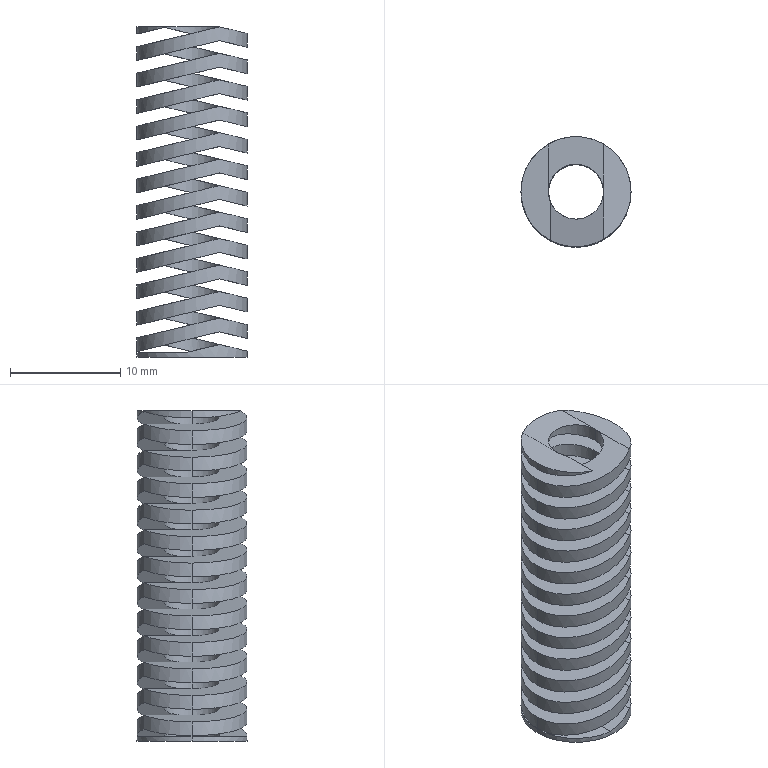Part | STEP file | 1 solid | 109 faces | box 10 x 10 x 30 mm | volume 930.907 mm3 | plane 55 | cylinder 54 | commonest cylinder face diameters 5 x27 10 x27